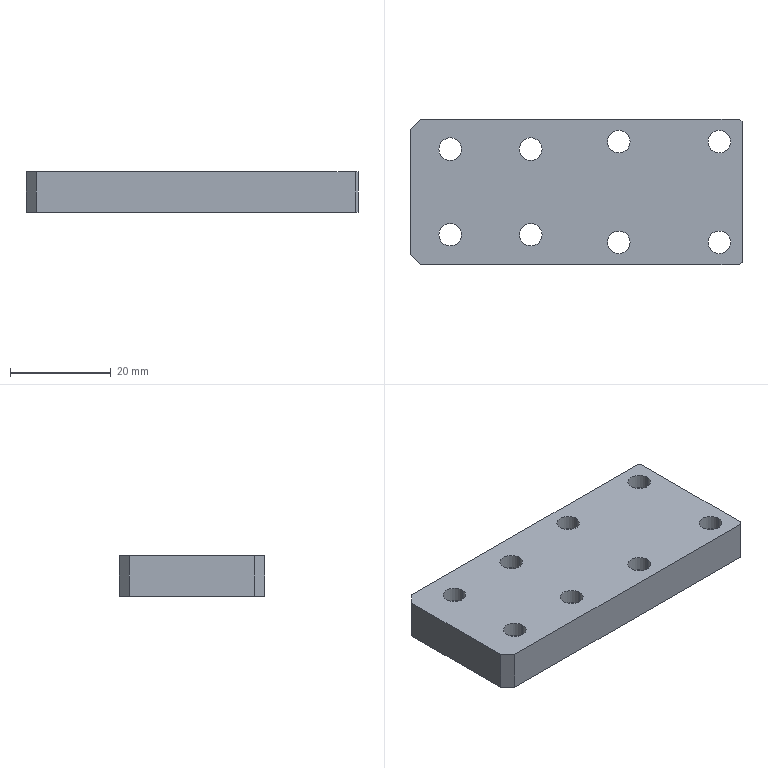Part | STEP file | ASND-0110-Body 1-12 | 1 solid | 50 faces | box 66 x 29 x 8 mm | volume 12885 mm3 | cylinder 32 | plane 18 | commonest cylinder face diameters 4.5 x16 8 x16